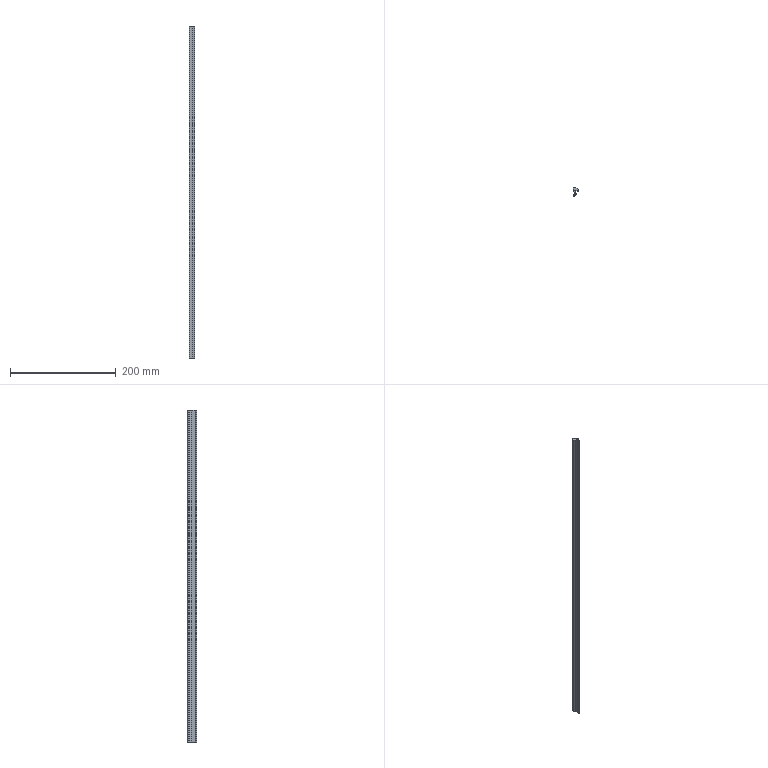Part | SolidWorks | features BaseBody 1, MoveFace 1 | 1 solid | 20 faces | box 10.8 x 17.5 x 627 mm | volume 49408 mm3 | cylinder 11 | plane 9 | commonest cylinder face diameters 1.6 x2 14 x2 0.4 x1 0.6 x1 0.8 x1 2.6 x1
STEP:
#1=CARTESIAN_POINT('',(-3.236,-11.055,527.));
#2=VERTEX_POINT('',#1);
#3=CARTESIAN_POINT('',(-4.3,-10.3,527.));
#4=VERTEX_POINT('',#3);
#5=CARTESIAN_POINT('',(-3.5,-10.3,527.));
#6=DIRECTION('',(0.,0.,-1.));
#7=DIRECTION('',(1.,0.,0.));
#8=AXIS2_PLACEMENT_3D('',#5,#6,#7);
#9=CIRCLE('',#8,0.8);
#10=EDGE_CURVE('',#2,#4,#9,.T.);
#11=ORIENTED_EDGE('',*,*,#10,.T.);
#12=CARTESIAN_POINT('',(-4.3,-10.3,-100.));
#13=VERTEX_POINT('',#12);
#14=CARTESIAN_POINT('',(-4.3,-10.3,-100.));
#15=DIRECTION('',(0.,0.,-1.));
#16=VECTOR('',#15,1000.);
#17=LINE('',#14,#16);
#18=EDGE_CURVE('',#4,#13,#17,.T.);
#19=ORIENTED_EDGE('',*,*,#18,.T.);
#20=CARTESIAN_POINT('',(-3.236,-11.055,-100.));
#21=VERTEX_POINT('',#20);
#22=CARTESIAN_POINT('',(-3.5,-10.3,-100.));
#23=DIRECTION('',(0.,0.,1.));
#24=DIRECTION('',(-1.,0.,0.));
#25=AXIS2_PLACEMENT_3D('',#22,#23,#24);
#26=CIRCLE('',#25,0.8);
#27=EDGE_CURVE('',#13,#21,#26,.T.);
#28=ORIENTED_EDGE('',*,*,#27,.T.);
#29=CARTESIAN_POINT('',(-3.236,-11.055,-100.));
#30=DIRECTION('',(0.,0.,-1.));
#31=VECTOR('',#30,1000.);
#32=LINE('',#29,#31);
#33=EDGE_CURVE('',#2,#21,#32,.T.);
#34=ORIENTED_EDGE('',*,*,#33,.F.);
#35=EDGE_LOOP('',(#11,#19,#28,#34));
#36=FACE_OUTER_BOUND('',#35,.T.);
#37=CARTESIAN_POINT('',(-3.5,-10.3,-100.));
#38=DIRECTION('',(0.,0.,-1.));
#39=DIRECTION('',(-1.,0.,0.));
#40=AXIS2_PLACEMENT_3D('',#37,#38,#39);
#41=CYLINDRICAL_SURFACE('',#40,0.8);
#42=ADVANCED_FACE('',(#36),#41,.T.);
#43=CARTESIAN_POINT('',(1.184,-6.397,-100.));
#44=VERTEX_POINT('',#43);
#45=CARTESIAN_POINT('',(-5.702,-4.29,-100.));
#46=DIRECTION('',(0.,0.,1.));
#47=DIRECTION('',(-1.,0.,0.));
#48=AXIS2_PLACEMENT_3D('',#45,#46,#47);
#49=CIRCLE('',#48,7.201);
#50=EDGE_CURVE('',#21,#44,#49,.T.);
#51=ORIENTED_EDGE('',*,*,#50,.T.);
#52=CARTESIAN_POINT('',(1.184,-6.397,527.));
#53=VERTEX_POINT('',#52);
#54=CARTESIAN_POINT('',(1.184,-6.397,-100.));
#55=DIRECTION('',(0.,0.,1.));
#56=VECTOR('',#55,1000.);
#57=LINE('',#54,#56);
#58=EDGE_CURVE('',#44,#53,#57,.T.);
#59=ORIENTED_EDGE('',*,*,#58,.T.);
#60=CARTESIAN_POINT('',(-5.702,-4.29,527.));
#61=DIRECTION('',(0.,0.,-1.));
#62=DIRECTION('',(1.,0.,0.));
#63=AXIS2_PLACEMENT_3D('',#60,#61,#62);
#64=CIRCLE('',#63,7.201);
#65=EDGE_CURVE('',#53,#2,#64,.T.);
#66=ORIENTED_EDGE('',*,*,#65,.T.);
#67=ORIENTED_EDGE('',*,*,#33,.T.);
#68=EDGE_LOOP('',(#51,#59,#66,#67));
#69=FACE_OUTER_BOUND('',#68,.T.);
#70=CARTESIAN_POINT('',(-5.702,-4.29,-100.));
#71=DIRECTION('',(0.,0.,-1.));
#72=DIRECTION('',(-1.,0.,0.));
#73=AXIS2_PLACEMENT_3D('',#70,#71,#72);
#74=CYLINDRICAL_SURFACE('',#73,7.201);
#75=ADVANCED_FACE('',(#69),#74,.T.);
#76=CARTESIAN_POINT('',(0.9,-6.,-100.));
#77=VERTEX_POINT('',#76);
#78=CARTESIAN_POINT('',(0.9,-6.3,-100.));
#79=DIRECTION('',(0.,0.,1.));
#80=DIRECTION('',(-1.,0.,0.));
#81=AXIS2_PLACEMENT_3D('',#78,#79,#80);
#82=CIRCLE('',#81,0.3);
#83=EDGE_CURVE('',#44,#77,#82,.T.);
#84=ORIENTED_EDGE('',*,*,#83,.T.);
#85=CARTESIAN_POINT('',(0.9,-6.,527.));
#86=VERTEX_POINT('',#85);
#87=CARTESIAN_POINT('',(0.9,-6.,-100.));
#88=DIRECTION('',(0.,0.,1.));
#89=VECTOR('',#88,1000.);
#90=LINE('',#87,#89);
#91=EDGE_CURVE('',#77,#86,#90,.T.);
#92=ORIENTED_EDGE('',*,*,#91,.T.);
#93=CARTESIAN_POINT('',(0.9,-6.3,527.));
#94=DIRECTION('',(0.,0.,-1.));
#95=DIRECTION('',(1.,0.,0.));
#96=AXIS2_PLACEMENT_3D('',#93,#94,#95);
#97=CIRCLE('',#96,0.3);
#98=EDGE_CURVE('',#86,#53,#97,.T.);
#99=ORIENTED_EDGE('',*,*,#98,.T.);
#100=ORIENTED_EDGE('',*,*,#58,.F.);
#101=EDGE_LOOP('',(#84,#92,#99,#100));
#102=FACE_OUTER_BOUND('',#101,.T.);
#103=CARTESIAN_POINT('',(0.9,-6.3,-100.));
#104=DIRECTION('',(0.,0.,-1.));
#105=DIRECTION('',(-1.,0.,0.));
#106=AXIS2_PLACEMENT_3D('',#103,#104,#105);
#107=CYLINDRICAL_SURFACE('',#106,0.3);
#108=ADVANCED_FACE('',(#102),#107,.T.);
#109=CARTESIAN_POINT('',(-2.5,-0.5,-100.));
#110=VERTEX_POINT('',#109);
#111=CARTESIAN_POINT('',(-2.5,-6.153,-100.));
#112=VERTEX_POINT('',#111);
#113=CARTESIAN_POINT('',(-2.5,-6.397,-100.));
#114=DIRECTION('',(0.,-1.,0.));
#115=VECTOR('',#114,1000.);
#116=LINE('',#113,#115);
#117=EDGE_CURVE('',#110,#112,#116,.T.);
#118=ORIENTED_EDGE('',*,*,#117,.F.);
#119=CARTESIAN_POINT('',(-4.2,1.695,-100.));
#120=VERTEX_POINT('',#119);
#121=CARTESIAN_POINT('',(-1.701,1.875,-100.));
#122=DIRECTION('',(0.,0.,1.));
#123=DIRECTION('',(-1.,0.,0.));
#124=AXIS2_PLACEMENT_3D('',#121,#122,#123);
#125=CIRCLE('',#124,2.506);
#126=EDGE_CURVE('',#120,#110,#125,.T.);
#127=ORIENTED_EDGE('',*,*,#126,.F.);
#128=CARTESIAN_POINT('',(-4.2,5.1,-100.));
#129=VERTEX_POINT('',#128);
#130=CARTESIAN_POINT('',(-4.2,-6.397,-100.));
#131=DIRECTION('',(0.,-1.,0.));
#132=VECTOR('',#131,1000.);
#133=LINE('',#130,#132);
#134=EDGE_CURVE('',#129,#120,#133,.T.);
#135=ORIENTED_EDGE('',*,*,#134,.F.);
#136=CARTESIAN_POINT('',(-2.892,6.4,-100.));
#137=VERTEX_POINT('',#136);
#138=CARTESIAN_POINT('',(-2.9,5.1,-100.));
#139=DIRECTION('',(0.,0.,1.));
#140=DIRECTION('',(-1.,0.,0.));
#141=AXIS2_PLACEMENT_3D('',#138,#139,#140);
#142=CIRCLE('',#141,1.3);
#143=EDGE_CURVE('',#137,#129,#142,.T.);
#144=ORIENTED_EDGE('',*,*,#143,.F.);
#145=CARTESIAN_POINT('',(0.5,5.5,-100.));
#146=VERTEX_POINT('',#145);
#147=CARTESIAN_POINT('',(-2.934,-0.5999,-100.));
#148=DIRECTION('',(0.,0.,1.));
#149=DIRECTION('',(-1.,0.,0.));
#150=AXIS2_PLACEMENT_3D('',#147,#148,#149);
#151=CIRCLE('',#150,7.);
#152=EDGE_CURVE('',#146,#137,#151,.T.);
#153=ORIENTED_EDGE('',*,*,#152,.F.);
#154=CARTESIAN_POINT('',(5.5,1.7,-100.));
#155=VERTEX_POINT('',#154);
#156=CARTESIAN_POINT('',(5.5,1.7,-100.));
#157=DIRECTION('',(-0.7962,0.6051,0.));
#158=VECTOR('',#157,1000.);
#159=LINE('',#156,#158);
#160=EDGE_CURVE('',#155,#146,#159,.T.);
#161=ORIENTED_EDGE('',*,*,#160,.F.);
#162=CARTESIAN_POINT('',(6.458,-0.2215,-100.));
#163=VERTEX_POINT('',#162);
#164=CARTESIAN_POINT('',(6.458,-0.2215,-100.));
#165=DIRECTION('',(-0.4462,0.8949,0.));
#166=VECTOR('',#165,1000.);
#167=LINE('',#164,#166);
#168=EDGE_CURVE('',#163,#155,#167,.T.);
#169=ORIENTED_EDGE('',*,*,#168,.F.);
#170=CARTESIAN_POINT('',(5.895,-0.7433,-100.));
#171=VERTEX_POINT('',#170);
#172=CARTESIAN_POINT('',(6.1,-0.4,-100.));
#173=DIRECTION('',(0.,0.,1.));
#174=DIRECTION('',(-1.,0.,0.));
#175=AXIS2_PLACEMENT_3D('',#172,#173,#174);
#176=CIRCLE('',#175,0.4);
#177=EDGE_CURVE('',#171,#163,#176,.T.);
#178=ORIENTED_EDGE('',*,*,#177,.F.);
#179=CARTESIAN_POINT('',(3.,0.,-100.));
#180=VERTEX_POINT('',#179);
#181=CARTESIAN_POINT('',(2.746,-6.995,-100.));
#182=DIRECTION('',(0.,0.,-1.));
#183=DIRECTION('',(-1.,0.,0.));
#184=AXIS2_PLACEMENT_3D('',#181,#182,#183);
#185=CIRCLE('',#184,7.);
#186=EDGE_CURVE('',#180,#171,#185,.T.);
#187=ORIENTED_EDGE('',*,*,#186,.F.);
#188=CARTESIAN_POINT('',(0.,0.,-100.));
#189=VERTEX_POINT('',#188);
#190=CARTESIAN_POINT('',(-6.814,0.,-100.));
#191=DIRECTION('',(1.,0.,0.));
#192=VECTOR('',#191,1000.);
#193=LINE('',#190,#192);
#194=EDGE_CURVE('',#189,#180,#193,.T.);
#195=ORIENTED_EDGE('',*,*,#194,.F.);
#196=CARTESIAN_POINT('',(0.,-5.8,-100.));
#197=VERTEX_POINT('',#196);
#198=CARTESIAN_POINT('',(0.,-6.397,-100.));
#199=DIRECTION('',(0.,1.,0.));
#200=VECTOR('',#199,1000.);
#201=LINE('',#198,#200);
#202=EDGE_CURVE('',#197,#189,#201,.T.);
#203=ORIENTED_EDGE('',*,*,#202,.F.);
#204=CARTESIAN_POINT('',(0.2,-6.,-100.));
#205=VERTEX_POINT('',#204);
#206=CARTESIAN_POINT('',(0.2,-5.8,-100.));
#207=DIRECTION('',(0.,0.,1.));
#208=DIRECTION('',(-1.,0.,0.));
#209=AXIS2_PLACEMENT_3D('',#206,#207,#208);
#210=CIRCLE('',#209,0.2);
#211=EDGE_CURVE('',#197,#205,#210,.T.);
#212=ORIENTED_EDGE('',*,*,#211,.T.);
#213=CARTESIAN_POINT('',(-6.814,-6.,-100.));
#214=DIRECTION('',(-1.,0.,0.));
#215=VECTOR('',#214,1000.);
#216=LINE('',#213,#215);
#217=EDGE_CURVE('',#77,#205,#216,.T.);
#218=ORIENTED_EDGE('',*,*,#217,.F.);
#219=ORIENTED_EDGE('',*,*,#83,.F.);
#220=ORIENTED_EDGE('',*,*,#50,.F.);
#221=ORIENTED_EDGE('',*,*,#27,.F.);
#222=CARTESIAN_POINT('',(-3.998,-9.674,-100.));
#223=VERTEX_POINT('',#222);
#224=CARTESIAN_POINT('',(-3.5,-10.3,-100.));
#225=DIRECTION('',(0.,0.,1.));
#226=DIRECTION('',(-1.,0.,0.));
#227=AXIS2_PLACEMENT_3D('',#224,#225,#226);
#228=CIRCLE('',#227,0.8);
#229=EDGE_CURVE('',#223,#13,#228,.T.);
#230=ORIENTED_EDGE('',*,*,#229,.F.);
#231=CARTESIAN_POINT('',(-6.814,-6.397,-100.));
#232=DIRECTION('',(0.,0.,-1.));
#233=DIRECTION('',(-1.,0.,0.));
#234=AXIS2_PLACEMENT_3D('',#231,#232,#233);
#235=CIRCLE('',#234,4.321);
#236=EDGE_CURVE('',#112,#223,#235,.T.);
#237=ORIENTED_EDGE('',*,*,#236,.F.);
#238=EDGE_LOOP('',(#118,#127,#135,#144,#153,#161,#169,#178,#187,#195,#203,#212,#218,#219,#220,#221,#230,#237));
#239=FACE_OUTER_BOUND('',#238,.T.);
#240=CARTESIAN_POINT('',(-6.814,-6.397,-100.));
#241=DIRECTION('',(0.,0.,1.));
#242=DIRECTION('',(1.,0.,0.));
#243=AXIS2_PLACEMENT_3D('',#240,#241,#242);
#244=PLANE('',#243);
#245=ADVANCED_FACE('',(#239),#244,.F.);
#246=ORIENTED_EDGE('',*,*,#18,.F.);
#247=CARTESIAN_POINT('',(-3.998,-9.674,527.));
#248=VERTEX_POINT('',#247);
#249=CARTESIAN_POINT('',(-3.5,-10.3,527.));
#250=DIRECTION('',(0.,0.,-1.));
#251=DIRECTION('',(1.,0.,0.));
#252=AXIS2_PLACEMENT_3D('',#249,#250,#251);
#253=CIRCLE('',#252,0.8);
#254=EDGE_CURVE('',#4,#248,#253,.T.);
#255=ORIENTED_EDGE('',*,*,#254,.T.);
#256=CARTESIAN_POINT('',(-3.998,-9.674,-100.));
#257=DIRECTION('',(0.,0.,-1.));
#258=VECTOR('',#257,1000.);
#259=LINE('',#256,#258);
#260=EDGE_CURVE('',#248,#223,#259,.T.);
#261=ORIENTED_EDGE('',*,*,#260,.T.);
#262=ORIENTED_EDGE('',*,*,#229,.T.);
#263=EDGE_LOOP('',(#246,#255,#261,#262));
#264=FACE_OUTER_BOUND('',#263,.T.);
#265=CARTESIAN_POINT('',(-3.5,-10.3,-100.));
#266=DIRECTION('',(0.,0.,-1.));
#267=DIRECTION('',(-1.,0.,0.));
#268=AXIS2_PLACEMENT_3D('',#265,#266,#267);
#269=CYLINDRICAL_SURFACE('',#268,0.8);
#270=ADVANCED_FACE('',(#264),#269,.T.);
#271=CARTESIAN_POINT('',(-4.2,1.695,527.));
#272=VERTEX_POINT('',#271);
#273=CARTESIAN_POINT('',(-2.5,-0.5,527.));
#274=VERTEX_POINT('',#273);
#275=CARTESIAN_POINT('',(-1.701,1.875,527.));
#276=DIRECTION('',(0.,0.,1.));
#277=DIRECTION('',(1.,0.,0.));
#278=AXIS2_PLACEMENT_3D('',#275,#276,#277);
#279=CIRCLE('',#278,2.506);
#280=EDGE_CURVE('',#272,#274,#279,.T.);
#281=ORIENTED_EDGE('',*,*,#280,.T.);
#282=CARTESIAN_POINT('',(-2.5,-6.153,527.));
#283=VERTEX_POINT('',#282);
#284=CARTESIAN_POINT('',(-2.5,-6.397,527.));
#285=DIRECTION('',(0.,-1.,0.));
#286=VECTOR('',#285,1000.);
#287=LINE('',#284,#286);
#288=EDGE_CURVE('',#274,#283,#287,.T.);
#289=ORIENTED_EDGE('',*,*,#288,.T.);
#290=CARTESIAN_POINT('',(-6.814,-6.397,527.));
#291=DIRECTION('',(0.,0.,-1.));
#292=DIRECTION('',(1.,0.,0.));
#293=AXIS2_PLACEMENT_3D('',#290,#291,#292);
#294=CIRCLE('',#293,4.321);
#295=EDGE_CURVE('',#283,#248,#294,.T.);
#296=ORIENTED_EDGE('',*,*,#295,.T.);
#297=ORIENTED_EDGE('',*,*,#254,.F.);
#298=ORIENTED_EDGE('',*,*,#10,.F.);
#299=ORIENTED_EDGE('',*,*,#65,.F.);
#300=ORIENTED_EDGE('',*,*,#98,.F.);
#301=CARTESIAN_POINT('',(0.2,-6.,527.));
#302=VERTEX_POINT('',#301);
#303=CARTESIAN_POINT('',(-6.814,-6.,527.));
#304=DIRECTION('',(-1.,0.,0.));
#305=VECTOR('',#304,1000.);
#306=LINE('',#303,#305);
#307=EDGE_CURVE('',#86,#302,#306,.T.);
#308=ORIENTED_EDGE('',*,*,#307,.T.);
#309=CARTESIAN_POINT('',(0.,-5.8,527.));
#310=VERTEX_POINT('',#309);
#311=CARTESIAN_POINT('',(0.2,-5.8,527.));
#312=DIRECTION('',(0.,0.,-1.));
#313=DIRECTION('',(1.,0.,0.));
#314=AXIS2_PLACEMENT_3D('',#311,#312,#313);
#315=CIRCLE('',#314,0.2);
#316=EDGE_CURVE('',#302,#310,#315,.T.);
#317=ORIENTED_EDGE('',*,*,#316,.T.);
#318=CARTESIAN_POINT('',(0.,0.,527.));
#319=VERTEX_POINT('',#318);
#320=CARTESIAN_POINT('',(0.,-6.397,527.));
#321=DIRECTION('',(0.,1.,0.));
#322=VECTOR('',#321,1000.);
#323=LINE('',#320,#322);
#324=EDGE_CURVE('',#310,#319,#323,.T.);
#325=ORIENTED_EDGE('',*,*,#324,.T.);
#326=CARTESIAN_POINT('',(3.,0.,527.));
#327=VERTEX_POINT('',#326);
#328=CARTESIAN_POINT('',(-6.814,0.,527.));
#329=DIRECTION('',(1.,0.,0.));
#330=VECTOR('',#329,1000.);
#331=LINE('',#328,#330);
#332=EDGE_CURVE('',#319,#327,#331,.T.);
#333=ORIENTED_EDGE('',*,*,#332,.T.);
#334=CARTESIAN_POINT('',(5.895,-0.7433,527.));
#335=VERTEX_POINT('',#334);
#336=CARTESIAN_POINT('',(2.746,-6.995,527.));
#337=DIRECTION('',(0.,0.,-1.));
#338=DIRECTION('',(1.,0.,0.));
#339=AXIS2_PLACEMENT_3D('',#336,#337,#338);
#340=CIRCLE('',#339,7.);
#341=EDGE_CURVE('',#327,#335,#340,.T.);
#342=ORIENTED_EDGE('',*,*,#341,.T.);
#343=CARTESIAN_POINT('',(6.458,-0.2215,527.));
#344=VERTEX_POINT('',#343);
#345=CARTESIAN_POINT('',(6.1,-0.4,527.));
#346=DIRECTION('',(0.,0.,-1.));
#347=DIRECTION('',(1.,0.,0.));
#348=AXIS2_PLACEMENT_3D('',#345,#346,#347);
#349=CIRCLE('',#348,0.4);
#350=EDGE_CURVE('',#344,#335,#349,.T.);
#351=ORIENTED_EDGE('',*,*,#350,.F.);
#352=CARTESIAN_POINT('',(5.5,1.7,527.));
#353=VERTEX_POINT('',#352);
#354=CARTESIAN_POINT('',(6.282,0.1323,527.));
#355=DIRECTION('',(-0.4462,0.8949,0.));
#356=VECTOR('',#355,1000.);
#357=LINE('',#354,#356);
#358=EDGE_CURVE('',#344,#353,#357,.T.);
#359=ORIENTED_EDGE('',*,*,#358,.T.);
#360=CARTESIAN_POINT('',(0.5,5.5,527.));
#361=VERTEX_POINT('',#360);
#362=CARTESIAN_POINT('',(1.595,4.668,527.));
#363=DIRECTION('',(-0.7962,0.6051,0.));
#364=VECTOR('',#363,1000.);
#365=LINE('',#362,#364);
#366=EDGE_CURVE('',#353,#361,#365,.T.);
#367=ORIENTED_EDGE('',*,*,#366,.T.);
#368=CARTESIAN_POINT('',(-2.892,6.4,527.));
#369=VERTEX_POINT('',#368);
#370=CARTESIAN_POINT('',(-2.934,-0.5999,527.));
#371=DIRECTION('',(0.,0.,1.));
#372=DIRECTION('',(1.,0.,0.));
#373=AXIS2_PLACEMENT_3D('',#370,#371,#372);
#374=CIRCLE('',#373,7.);
#375=EDGE_CURVE('',#361,#369,#374,.T.);
#376=ORIENTED_EDGE('',*,*,#375,.T.);
#377=CARTESIAN_POINT('',(-4.2,5.1,527.));
#378=VERTEX_POINT('',#377);
#379=CARTESIAN_POINT('',(-2.9,5.1,527.));
#380=DIRECTION('',(0.,0.,1.));
#381=DIRECTION('',(1.,0.,0.));
#382=AXIS2_PLACEMENT_3D('',#379,#380,#381);
#383=CIRCLE('',#382,1.3);
#384=EDGE_CURVE('',#369,#378,#383,.T.);
#385=ORIENTED_EDGE('',*,*,#384,.T.);
#386=CARTESIAN_POINT('',(-4.2,-6.397,527.));
#387=DIRECTION('',(0.,-1.,0.));
#388=VECTOR('',#387,1000.);
#389=LINE('',#386,#388);
#390=EDGE_CURVE('',#378,#272,#389,.T.);
#391=ORIENTED_EDGE('',*,*,#390,.T.);
#392=EDGE_LOOP('',(#281,#289,#296,#297,#298,#299,#300,#308,#317,#325,#333,#342,#351,#359,#367,#376,#385,#391));
#393=FACE_OUTER_BOUND('',#392,.T.);
#394=CARTESIAN_POINT('',(-6.814,-6.397,527.));
#395=DIRECTION('',(0.,0.,1.));
#396=DIRECTION('',(1.,0.,0.));
#397=AXIS2_PLACEMENT_3D('',#394,#395,#396);
#398=PLANE('',#397);
#399=ADVANCED_FACE('',(#393),#398,.T.);
#400=ORIENTED_EDGE('',*,*,#217,.T.);
#401=CARTESIAN_POINT('',(0.2,-6.,-100.));
#402=DIRECTION('',(0.,0.,1.));
#403=VECTOR('',#402,1000.);
#404=LINE('',#401,#403);
#405=EDGE_CURVE('',#205,#302,#404,.T.);
#406=ORIENTED_EDGE('',*,*,#405,.T.);
#407=ORIENTED_EDGE('',*,*,#307,.F.);
#408=ORIENTED_EDGE('',*,*,#91,.F.);
#409=EDGE_LOOP('',(#400,#406,#407,#408));
#410=FACE_OUTER_BOUND('',#409,.T.);
#411=CARTESIAN_POINT('',(0.9,-6.,-100.));
#412=DIRECTION('',(0.,1.,0.));
#413=DIRECTION('',(0.,0.,1.));
#414=AXIS2_PLACEMENT_3D('',#411,#412,#413);
#415=PLANE('',#414);
#416=ADVANCED_FACE('',(#410),#415,.T.);
#417=CARTESIAN_POINT('',(-2.5,-6.153,-100.));
#418=DIRECTION('',(0.,0.,1.));
#419=VECTOR('',#418,1000.);
#420=LINE('',#417,#419);
#421=EDGE_CURVE('',#112,#283,#420,.T.);
#422=ORIENTED_EDGE('',*,*,#421,.F.);
#423=ORIENTED_EDGE('',*,*,#236,.T.);
#424=ORIENTED_EDGE('',*,*,#260,.F.);
#425=ORIENTED_EDGE('',*,*,#295,.F.);
#426=EDGE_LOOP('',(#422,#423,#424,#425));
#427=FACE_OUTER_BOUND('',#426,.T.);
#428=CARTESIAN_POINT('',(-6.814,-6.397,-100.));
#429=DIRECTION('',(0.,0.,-1.));
#430=DIRECTION('',(-1.,0.,0.));
#431=AXIS2_PLACEMENT_3D('',#428,#429,#430);
#432=CYLINDRICAL_SURFACE('',#431,4.321);
#433=ADVANCED_FACE('',(#427),#432,.F.);
#434=ORIENTED_EDGE('',*,*,#117,.T.);
#435=ORIENTED_EDGE('',*,*,#421,.T.);
#436=ORIENTED_EDGE('',*,*,#288,.F.);
#437=CARTESIAN_POINT('',(-2.5,-0.5,-100.));
#438=DIRECTION('',(0.,0.,-1.));
#439=VECTOR('',#438,1000.);
#440=LINE('',#437,#439);
#441=EDGE_CURVE('',#274,#110,#440,.T.);
#442=ORIENTED_EDGE('',*,*,#441,.T.);
#443=EDGE_LOOP('',(#434,#435,#436,#442));
#444=FACE_OUTER_BOUND('',#443,.T.);
#445=CARTESIAN_POINT('',(-2.5,-0.5,-100.));
#446=DIRECTION('',(-1.,0.,0.));
#447=DIRECTION('',(0.,0.,1.));
#448=AXIS2_PLACEMENT_3D('',#445,#446,#447);
#449=PLANE('',#448);
#450=ADVANCED_FACE('',(#444),#449,.T.);
#451=ORIENTED_EDGE('',*,*,#126,.T.);
#452=ORIENTED_EDGE('',*,*,#441,.F.);
#453=ORIENTED_EDGE('',*,*,#280,.F.);
#454=CARTESIAN_POINT('',(-4.2,1.695,-100.));
#455=DIRECTION('',(0.,0.,-1.));
#456=VECTOR('',#455,1000.);
#457=LINE('',#454,#456);
#458=EDGE_CURVE('',#272,#120,#457,.T.);
#459=ORIENTED_EDGE('',*,*,#458,.T.);
#460=EDGE_LOOP('',(#451,#452,#453,#459));
#461=FACE_OUTER_BOUND('',#460,.T.);
#462=CARTESIAN_POINT('',(-1.701,1.875,-100.));
#463=DIRECTION('',(0.,0.,-1.));
#464=DIRECTION('',(-1.,0.,0.));
#465=AXIS2_PLACEMENT_3D('',#462,#463,#464);
#466=CYLINDRICAL_SURFACE('',#465,2.506);
#467=ADVANCED_FACE('',(#461),#466,.T.);
#468=ORIENTED_EDGE('',*,*,#134,.T.);
#469=ORIENTED_EDGE('',*,*,#458,.F.);
#470=ORIENTED_EDGE('',*,*,#390,.F.);
#471=CARTESIAN_POINT('',(-4.2,5.1,-100.));
#472=DIRECTION('',(0.,0.,-1.));
#473=VECTOR('',#472,1000.);
#474=LINE('',#471,#473);
#475=EDGE_CURVE('',#378,#129,#474,.T.);
#476=ORIENTED_EDGE('',*,*,#475,.T.);
#477=EDGE_LOOP('',(#468,#469,#470,#476));
#478=FACE_OUTER_BOUND('',#477,.T.);
#479=CARTESIAN_POINT('',(-4.2,5.1,-100.));
#480=DIRECTION('',(-1.,0.,0.));
#481=DIRECTION('',(0.,0.,1.));
#482=AXIS2_PLACEMENT_3D('',#479,#480,#481);
#483=PLANE('',#482);
#484=ADVANCED_FACE('',(#478),#483,.T.);
#485=ORIENTED_EDGE('',*,*,#143,.T.);
#486=ORIENTED_EDGE('',*,*,#475,.F.);
#487=ORIENTED_EDGE('',*,*,#384,.F.);
#488=CARTESIAN_POINT('',(-2.892,6.4,-100.));
#489=DIRECTION('',(0.,0.,-1.));
#490=VECTOR('',#489,1000.);
#491=LINE('',#488,#490);
#492=EDGE_CURVE('',#369,#137,#491,.T.);
#493=ORIENTED_EDGE('',*,*,#492,.T.);
#494=EDGE_LOOP('',(#485,#486,#487,#493));
#495=FACE_OUTER_BOUND('',#494,.T.);
#496=CARTESIAN_POINT('',(-2.9,5.1,-100.));
#497=DIRECTION('',(0.,0.,-1.));
#498=DIRECTION('',(-1.,0.,0.));
#499=AXIS2_PLACEMENT_3D('',#496,#497,#498);
#500=CYLINDRICAL_SURFACE('',#499,1.3);
#501=ADVANCED_FACE('',(#495),#500,.T.);
#502=ORIENTED_EDGE('',*,*,#152,.T.);
#503=ORIENTED_EDGE('',*,*,#492,.F.);
#504=ORIENTED_EDGE('',*,*,#375,.F.);
#505=CARTESIAN_POINT('',(0.5,5.5,-100.));
#506=DIRECTION('',(0.,0.,-1.));
#507=VECTOR('',#506,1000.);
#508=LINE('',#505,#507);
#509=EDGE_CURVE('',#361,#146,#508,.T.);
#510=ORIENTED_EDGE('',*,*,#509,.T.);
#511=EDGE_LOOP('',(#502,#503,#504,#510));
#512=FACE_OUTER_BOUND('',#511,.T.);
#513=CARTESIAN_POINT('',(-2.934,-0.5999,-100.));
#514=DIRECTION('',(0.,0.,-1.));
#515=DIRECTION('',(-1.,0.,0.));
#516=AXIS2_PLACEMENT_3D('',#513,#514,#515);
#517=CYLINDRICAL_SURFACE('',#516,7.);
#518=ADVANCED_FACE('',(#512),#517,.T.);
#519=ORIENTED_EDGE('',*,*,#160,.T.);
#520=ORIENTED_EDGE('',*,*,#509,.F.);
#521=ORIENTED_EDGE('',*,*,#366,.F.);
#522=CARTESIAN_POINT('',(5.5,1.7,-100.));
#523=DIRECTION('',(0.,0.,-1.));
#524=VECTOR('',#523,1000.);
#525=LINE('',#522,#524);
#526=EDGE_CURVE('',#353,#155,#525,.T.);
#527=ORIENTED_EDGE('',*,*,#526,.T.);
#528=EDGE_LOOP('',(#519,#520,#521,#527));
#529=FACE_OUTER_BOUND('',#528,.T.);
#530=CARTESIAN_POINT('',(5.5,1.7,-100.));
#531=DIRECTION('',(0.6051,0.7962,0.));
#532=DIRECTION('',(-0.7962,0.6051,0.));
#533=AXIS2_PLACEMENT_3D('',#530,#531,#532);
#534=PLANE('',#533);
#535=ADVANCED_FACE('',(#529),#534,.T.);
#536=ORIENTED_EDGE('',*,*,#168,.T.);
#537=ORIENTED_EDGE('',*,*,#526,.F.);
#538=ORIENTED_EDGE('',*,*,#358,.F.);
#539=CARTESIAN_POINT('',(6.458,-0.2215,-100.));
#540=DIRECTION('',(0.,0.,-1.));
#541=VECTOR('',#540,1000.);
#542=LINE('',#539,#541);
#543=EDGE_CURVE('',#344,#163,#542,.T.);
#544=ORIENTED_EDGE('',*,*,#543,.T.);
#545=EDGE_LOOP('',(#536,#537,#538,#544));
#546=FACE_OUTER_BOUND('',#545,.T.);
#547=CARTESIAN_POINT('',(6.458,-0.2215,-100.));
#548=DIRECTION('',(0.8949,0.4462,0.));
#549=DIRECTION('',(-0.4462,0.8949,0.));
#550=AXIS2_PLACEMENT_3D('',#547,#548,#549);
#551=PLANE('',#550);
#552=ADVANCED_FACE('',(#546),#551,.T.);
#553=CARTESIAN_POINT('',(3.,0.,-100.));
#554=DIRECTION('',(0.,0.,1.));
#555=VECTOR('',#554,1000.);
#556=LINE('',#553,#555);
#557=EDGE_CURVE('',#180,#327,#556,.T.);
#558=ORIENTED_EDGE('',*,*,#557,.F.);
#559=ORIENTED_EDGE('',*,*,#186,.T.);
#560=CARTESIAN_POINT('',(5.895,-0.7433,-100.));
#561=DIRECTION('',(0.,0.,-1.));
#562=VECTOR('',#561,1000.);
#563=LINE('',#560,#562);
#564=EDGE_CURVE('',#335,#171,#563,.T.);
#565=ORIENTED_EDGE('',*,*,#564,.F.);
#566=ORIENTED_EDGE('',*,*,#341,.F.);
#567=EDGE_LOOP('',(#558,#559,#565,#566));
#568=FACE_OUTER_BOUND('',#567,.T.);
#569=CARTESIAN_POINT('',(2.746,-6.995,-100.));
#570=DIRECTION('',(0.,0.,-1.));
#571=DIRECTION('',(-1.,0.,0.));
#572=AXIS2_PLACEMENT_3D('',#569,#570,#571);
#573=CYLINDRICAL_SURFACE('',#572,7.);
#574=ADVANCED_FACE('',(#568),#573,.F.);
#575=ORIENTED_EDGE('',*,*,#194,.T.);
#576=ORIENTED_EDGE('',*,*,#557,.T.);
#577=ORIENTED_EDGE('',*,*,#332,.F.);
#578=CARTESIAN_POINT('',(0.,0.,-100.));
#579=DIRECTION('',(0.,0.,-1.));
#580=VECTOR('',#579,1000.);
#581=LINE('',#578,#580);
#582=EDGE_CURVE('',#319,#189,#581,.T.);
#583=ORIENTED_EDGE('',*,*,#582,.T.);
#584=EDGE_LOOP('',(#575,#576,#577,#583));
#585=FACE_OUTER_BOUND('',#584,.T.);
#586=CARTESIAN_POINT('',(0.,0.,-100.));
#587=DIRECTION('',(0.,-1.,0.));
#588=DIRECTION('',(0.,0.,-1.));
#589=AXIS2_PLACEMENT_3D('',#586,#587,#588);
#590=PLANE('',#589);
#591=ADVANCED_FACE('',(#585),#590,.T.);
#592=ORIENTED_EDGE('',*,*,#202,.T.);
#593=ORIENTED_EDGE('',*,*,#582,.F.);
#594=ORIENTED_EDGE('',*,*,#324,.F.);
#595=CARTESIAN_POINT('',(0.,-5.8,-100.));
#596=DIRECTION('',(0.,0.,-1.));
#597=VECTOR('',#596,1000.);
#598=LINE('',#595,#597);
#599=EDGE_CURVE('',#310,#197,#598,.T.);
#600=ORIENTED_EDGE('',*,*,#599,.T.);
#601=EDGE_LOOP('',(#592,#593,#594,#600));
#602=FACE_OUTER_BOUND('',#601,.T.);
#603=CARTESIAN_POINT('',(0.,-5.8,-100.));
#604=DIRECTION('',(1.,0.,0.));
#605=DIRECTION('',(0.,0.,-1.));
#606=AXIS2_PLACEMENT_3D('',#603,#604,#605);
#607=PLANE('',#606);
#608=ADVANCED_FACE('',(#602),#607,.T.);
#609=ORIENTED_EDGE('',*,*,#405,.F.);
#610=ORIENTED_EDGE('',*,*,#211,.F.);
#611=ORIENTED_EDGE('',*,*,#599,.F.);
#612=ORIENTED_EDGE('',*,*,#316,.F.);
#613=EDGE_LOOP('',(#609,#610,#611,#612));
#614=FACE_OUTER_BOUND('',#613,.T.);
#615=CARTESIAN_POINT('',(0.2,-5.8,-100.));
#616=DIRECTION('',(0.,0.,-1.));
#617=DIRECTION('',(-1.,0.,0.));
#618=AXIS2_PLACEMENT_3D('',#615,#616,#617);
#619=CYLINDRICAL_SURFACE('',#618,0.2);
#620=ADVANCED_FACE('',(#614),#619,.F.);
#621=ORIENTED_EDGE('',*,*,#177,.T.);
#622=ORIENTED_EDGE('',*,*,#543,.F.);
#623=ORIENTED_EDGE('',*,*,#350,.T.);
#624=ORIENTED_EDGE('',*,*,#564,.T.);
#625=EDGE_LOOP('',(#621,#622,#623,#624));
#626=FACE_OUTER_BOUND('',#625,.T.);
#627=CARTESIAN_POINT('',(6.1,-0.4,-100.));
#628=DIRECTION('',(0.,0.,-1.));
#629=DIRECTION('',(-1.,0.,0.));
#630=AXIS2_PLACEMENT_3D('',#627,#628,#629);
#631=CYLINDRICAL_SURFACE('',#630,0.4);
#632=ADVANCED_FACE('',(#626),#631,.T.);
#633=CLOSED_SHELL('',(#42,#75,#108,#245,#270,#399,#416,#433,#450,#467,#484,#501,#518,#535,#552,#574,#591,#608,#620,#632));
#634=MANIFOLD_SOLID_BREP('',#633);
#635=CARTESIAN_POINT('',(0.,0.,0.));
#636=DIRECTION('',(0.,0.,1.));
#637=DIRECTION('',(1.,0.,0.));
#638=AXIS2_PLACEMENT_3D('',#635,#636,#637);
#639=(LENGTH_UNIT()NAMED_UNIT(*)SI_UNIT(.MILLI.,.METRE.));
#640=UNCERTAINTY_MEASURE_WITH_UNIT(LENGTH_MEASURE(0.00001),#639,'','');
#641=(NAMED_UNIT(*)PLANE_ANGLE_UNIT()SI_UNIT($,.RADIAN.));
#642=(NAMED_UNIT(*)SI_UNIT($,.STERADIAN.)SOLID_ANGLE_UNIT());
#643=(GEOMETRIC_REPRESENTATION_CONTEXT(3)GLOBAL_UNCERTAINTY_ASSIGNED_CONTEXT((#640))GLOBAL_UNIT_ASSIGNED_CONTEXT((#639,#641,#642))REPRESENTATION_CONTEXT('',''));
#644=ADVANCED_BREP_SHAPE_REPRESENTATION('',(#634,#638),#643);